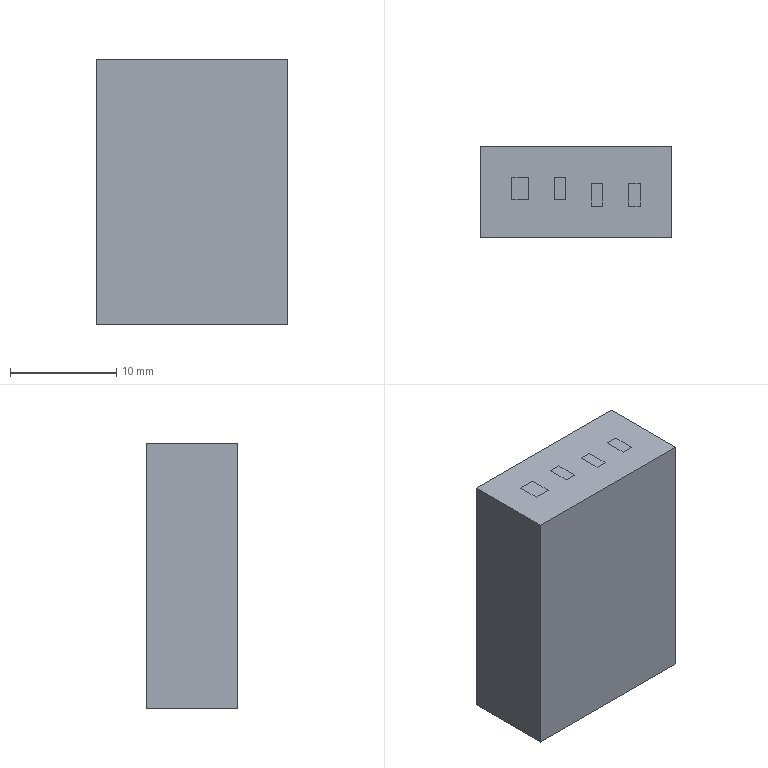Part | NX | features BREP 2 | 2 solids | 48 faces | box 18.008 x 8.593 x 25 mm | volume 6543 mm3 | plane 48
STEP:
#1=CARTESIAN_POINT('',(-9.004,-4.296,-25.6));
#2=VERTEX_POINT('',#1);
#3=CARTESIAN_POINT('',(-9.004,4.296,-25.6));
#4=VERTEX_POINT('',#3);
#5=CARTESIAN_POINT('',(-9.004,-4.296,-25.6));
#6=DIRECTION('',(0.,1.,0.));
#7=VECTOR('',#6,1000.);
#8=LINE('',#5,#7);
#9=EDGE_CURVE('',#2,#4,#8,.T.);
#10=ORIENTED_EDGE('',*,*,#9,.T.);
#11=CARTESIAN_POINT('',(9.004,4.296,-25.6));
#12=VERTEX_POINT('',#11);
#13=CARTESIAN_POINT('',(-9.004,4.296,-25.6));
#14=DIRECTION('',(1.,0.,0.));
#15=VECTOR('',#14,1000.);
#16=LINE('',#13,#15);
#17=EDGE_CURVE('',#4,#12,#16,.T.);
#18=ORIENTED_EDGE('',*,*,#17,.T.);
#19=CARTESIAN_POINT('',(9.004,-4.296,-25.6));
#20=VERTEX_POINT('',#19);
#21=CARTESIAN_POINT('',(9.004,4.296,-25.6));
#22=DIRECTION('',(0.,-1.,0.));
#23=VECTOR('',#22,1000.);
#24=LINE('',#21,#23);
#25=EDGE_CURVE('',#12,#20,#24,.T.);
#26=ORIENTED_EDGE('',*,*,#25,.T.);
#27=CARTESIAN_POINT('',(9.004,-4.296,-25.6));
#28=DIRECTION('',(-1.,0.,0.));
#29=VECTOR('',#28,1000.);
#30=LINE('',#27,#29);
#31=EDGE_CURVE('',#20,#2,#30,.T.);
#32=ORIENTED_EDGE('',*,*,#31,.T.);
#33=EDGE_LOOP('',(#10,#18,#26,#32));
#34=FACE_BOUND('',#33,.T.);
#35=CARTESIAN_POINT('',(7.054,1.754,-25.6));
#36=VERTEX_POINT('',#35);
#37=CARTESIAN_POINT('',(3.934,1.754,-25.6));
#38=VERTEX_POINT('',#37);
#39=CARTESIAN_POINT('',(-5.046,1.754,-25.6));
#40=DIRECTION('',(-1.,0.,0.));
#41=VECTOR('',#40,1000.);
#42=LINE('',#39,#41);
#43=EDGE_CURVE('',#36,#38,#42,.T.);
#44=ORIENTED_EDGE('',*,*,#43,.T.);
#45=CARTESIAN_POINT('',(3.934,-2.346,-25.6));
#46=VERTEX_POINT('',#45);
#47=CARTESIAN_POINT('',(3.934,-10.383,-25.6));
#48=DIRECTION('',(0.,-1.,0.));
#49=VECTOR('',#48,1000.);
#50=LINE('',#47,#49);
#51=EDGE_CURVE('',#38,#46,#50,.T.);
#52=ORIENTED_EDGE('',*,*,#51,.T.);
#53=CARTESIAN_POINT('',(7.054,-2.346,-25.6));
#54=VERTEX_POINT('',#53);
#55=CARTESIAN_POINT('',(-5.046,-2.346,-25.6));
#56=DIRECTION('',(1.,0.,0.));
#57=VECTOR('',#56,1000.);
#58=LINE('',#55,#57);
#59=EDGE_CURVE('',#46,#54,#58,.T.);
#60=ORIENTED_EDGE('',*,*,#59,.T.);
#61=CARTESIAN_POINT('',(7.054,1.396,-25.6));
#62=DIRECTION('',(0.,1.,0.));
#63=VECTOR('',#62,1000.);
#64=LINE('',#61,#63);
#65=EDGE_CURVE('',#54,#36,#64,.T.);
#66=ORIENTED_EDGE('',*,*,#65,.T.);
#67=EDGE_LOOP('',(#44,#52,#60,#66));
#68=FACE_BOUND('',#67,.T.);
#69=CARTESIAN_POINT('',(3.534,1.754,-25.6));
#70=VERTEX_POINT('',#69);
#71=CARTESIAN_POINT('',(0.454,1.754,-25.6));
#72=VERTEX_POINT('',#71);
#73=CARTESIAN_POINT('',(-5.046,1.754,-25.6));
#74=DIRECTION('',(-1.,0.,0.));
#75=VECTOR('',#74,1000.);
#76=LINE('',#73,#75);
#77=EDGE_CURVE('',#70,#72,#76,.T.);
#78=ORIENTED_EDGE('',*,*,#77,.T.);
#79=CARTESIAN_POINT('',(0.454,-2.346,-25.6));
#80=VERTEX_POINT('',#79);
#81=CARTESIAN_POINT('',(0.454,-1.296,-25.6));
#82=DIRECTION('',(0.,-1.,0.));
#83=VECTOR('',#82,1000.);
#84=LINE('',#81,#83);
#85=EDGE_CURVE('',#72,#80,#84,.T.);
#86=ORIENTED_EDGE('',*,*,#85,.T.);
#87=CARTESIAN_POINT('',(3.534,-2.346,-25.6));
#88=VERTEX_POINT('',#87);
#89=CARTESIAN_POINT('',(-5.046,-2.346,-25.6));
#90=DIRECTION('',(1.,0.,0.));
#91=VECTOR('',#90,1000.);
#92=LINE('',#89,#91);
#93=EDGE_CURVE('',#80,#88,#92,.T.);
#94=ORIENTED_EDGE('',*,*,#93,.T.);
#95=CARTESIAN_POINT('',(3.534,1.396,-25.6));
#96=DIRECTION('',(0.,1.,0.));
#97=VECTOR('',#96,1000.);
#98=LINE('',#95,#97);
#99=EDGE_CURVE('',#88,#70,#98,.T.);
#100=ORIENTED_EDGE('',*,*,#99,.T.);
#101=EDGE_LOOP('',(#78,#86,#94,#100));
#102=FACE_BOUND('',#101,.T.);
#103=CARTESIAN_POINT('',(0.04599,-1.754,-25.6));
#104=VERTEX_POINT('',#103);
#105=CARTESIAN_POINT('',(0.04599,2.346,-25.6));
#106=VERTEX_POINT('',#105);
#107=CARTESIAN_POINT('',(0.04599,4.296,-25.6));
#108=DIRECTION('',(0.,1.,0.));
#109=VECTOR('',#108,1000.);
#110=LINE('',#107,#109);
#111=EDGE_CURVE('',#104,#106,#110,.T.);
#112=ORIENTED_EDGE('',*,*,#111,.T.);
#113=CARTESIAN_POINT('',(-3.054,2.346,-25.6));
#114=VERTEX_POINT('',#113);
#115=CARTESIAN_POINT('',(-5.046,2.346,-25.6));
#116=DIRECTION('',(-1.,0.,0.));
#117=VECTOR('',#116,1000.);
#118=LINE('',#115,#117);
#119=EDGE_CURVE('',#106,#114,#118,.T.);
#120=ORIENTED_EDGE('',*,*,#119,.T.);
#121=CARTESIAN_POINT('',(-3.054,-1.754,-25.6));
#122=VERTEX_POINT('',#121);
#123=CARTESIAN_POINT('',(-3.054,-1.296,-25.6));
#124=DIRECTION('',(0.,-1.,0.));
#125=VECTOR('',#124,1000.);
#126=LINE('',#123,#125);
#127=EDGE_CURVE('',#114,#122,#126,.T.);
#128=ORIENTED_EDGE('',*,*,#127,.T.);
#129=CARTESIAN_POINT('',(-5.046,-1.754,-25.6));
#130=DIRECTION('',(1.,0.,0.));
#131=VECTOR('',#130,1000.);
#132=LINE('',#129,#131);
#133=EDGE_CURVE('',#122,#104,#132,.T.);
#134=ORIENTED_EDGE('',*,*,#133,.T.);
#135=EDGE_LOOP('',(#112,#120,#128,#134));
#136=FACE_BOUND('',#135,.T.);
#137=CARTESIAN_POINT('',(-3.454,-1.754,-25.6));
#138=VERTEX_POINT('',#137);
#139=CARTESIAN_POINT('',(-3.454,2.346,-25.6));
#140=VERTEX_POINT('',#139);
#141=CARTESIAN_POINT('',(-3.454,4.296,-25.6));
#142=DIRECTION('',(0.,1.,0.));
#143=VECTOR('',#142,1000.);
#144=LINE('',#141,#143);
#145=EDGE_CURVE('',#138,#140,#144,.T.);
#146=ORIENTED_EDGE('',*,*,#145,.T.);
#147=CARTESIAN_POINT('',(-7.054,2.346,-25.6));
#148=VERTEX_POINT('',#147);
#149=CARTESIAN_POINT('',(-5.046,2.346,-25.6));
#150=DIRECTION('',(-1.,0.,0.));
#151=VECTOR('',#150,1000.);
#152=LINE('',#149,#151);
#153=EDGE_CURVE('',#140,#148,#152,.T.);
#154=ORIENTED_EDGE('',*,*,#153,.T.);
#155=CARTESIAN_POINT('',(-7.054,-1.754,-25.6));
#156=VERTEX_POINT('',#155);
#157=CARTESIAN_POINT('',(-7.054,-1.196,-25.6));
#158=DIRECTION('',(0.,-1.,0.));
#159=VECTOR('',#158,1000.);
#160=LINE('',#157,#159);
#161=EDGE_CURVE('',#148,#156,#160,.T.);
#162=ORIENTED_EDGE('',*,*,#161,.T.);
#163=CARTESIAN_POINT('',(-5.046,-1.754,-25.6));
#164=DIRECTION('',(1.,0.,0.));
#165=VECTOR('',#164,1000.);
#166=LINE('',#163,#165);
#167=EDGE_CURVE('',#156,#138,#166,.T.);
#168=ORIENTED_EDGE('',*,*,#167,.T.);
#169=EDGE_LOOP('',(#146,#154,#162,#168));
#170=FACE_BOUND('',#169,.T.);
#171=CARTESIAN_POINT('',(0.,0.,-25.6));
#172=DIRECTION('',(0.,0.,-1.));
#173=DIRECTION('',(1.,0.,0.));
#174=AXIS2_PLACEMENT_3D('',#171,#172,#173);
#175=PLANE('',#174);
#176=ADVANCED_FACE('',(#34,#68,#102,#136,#170),#175,.T.);
#177=CARTESIAN_POINT('',(-0.954,1.346,-0.6));
#178=VERTEX_POINT('',#177);
#179=CARTESIAN_POINT('',(-2.054,1.346,-0.6));
#180=VERTEX_POINT('',#179);
#181=CARTESIAN_POINT('',(-5.046,1.346,-0.6));
#182=DIRECTION('',(-1.,0.,0.));
#183=VECTOR('',#182,1000.);
#184=LINE('',#181,#183);
#185=EDGE_CURVE('',#178,#180,#184,.T.);
#186=ORIENTED_EDGE('',*,*,#185,.F.);
#187=CARTESIAN_POINT('',(-0.954,-0.7536,-0.6));
#188=VERTEX_POINT('',#187);
#189=CARTESIAN_POINT('',(-0.954,4.296,-0.6));
#190=DIRECTION('',(0.,1.,0.));
#191=VECTOR('',#190,1000.);
#192=LINE('',#189,#191);
#193=EDGE_CURVE('',#188,#178,#192,.T.);
#194=ORIENTED_EDGE('',*,*,#193,.F.);
#195=CARTESIAN_POINT('',(-2.054,-0.7536,-0.6));
#196=VERTEX_POINT('',#195);
#197=CARTESIAN_POINT('',(-5.046,-0.7536,-0.6));
#198=DIRECTION('',(1.,0.,0.));
#199=VECTOR('',#198,1000.);
#200=LINE('',#197,#199);
#201=EDGE_CURVE('',#196,#188,#200,.T.);
#202=ORIENTED_EDGE('',*,*,#201,.F.);
#203=CARTESIAN_POINT('',(-2.054,-1.296,-0.6));
#204=DIRECTION('',(0.,-1.,0.));
#205=VECTOR('',#204,1000.);
#206=LINE('',#203,#205);
#207=EDGE_CURVE('',#180,#196,#206,.T.);
#208=ORIENTED_EDGE('',*,*,#207,.F.);
#209=EDGE_LOOP('',(#186,#194,#202,#208));
#210=FACE_BOUND('',#209,.T.);
#211=CARTESIAN_POINT('',(-9.004,-4.296,-0.6));
#212=VERTEX_POINT('',#211);
#213=CARTESIAN_POINT('',(-9.004,4.296,-0.6));
#214=VERTEX_POINT('',#213);
#215=CARTESIAN_POINT('',(-9.004,-4.296,-0.6));
#216=DIRECTION('',(0.,1.,0.));
#217=VECTOR('',#216,1000.);
#218=LINE('',#215,#217);
#219=EDGE_CURVE('',#212,#214,#218,.T.);
#220=ORIENTED_EDGE('',*,*,#219,.F.);
#221=CARTESIAN_POINT('',(9.004,-4.296,-0.6));
#222=VERTEX_POINT('',#221);
#223=CARTESIAN_POINT('',(9.004,-4.296,-0.6));
#224=DIRECTION('',(-1.,0.,0.));
#225=VECTOR('',#224,1000.);
#226=LINE('',#223,#225);
#227=EDGE_CURVE('',#222,#212,#226,.T.);
#228=ORIENTED_EDGE('',*,*,#227,.F.);
#229=CARTESIAN_POINT('',(9.004,4.296,-0.6));
#230=VERTEX_POINT('',#229);
#231=CARTESIAN_POINT('',(9.004,4.296,-0.6));
#232=DIRECTION('',(0.,-1.,0.));
#233=VECTOR('',#232,1000.);
#234=LINE('',#231,#233);
#235=EDGE_CURVE('',#230,#222,#234,.T.);
#236=ORIENTED_EDGE('',*,*,#235,.F.);
#237=CARTESIAN_POINT('',(-9.004,4.296,-0.6));
#238=DIRECTION('',(1.,0.,0.));
#239=VECTOR('',#238,1000.);
#240=LINE('',#237,#239);
#241=EDGE_CURVE('',#214,#230,#240,.T.);
#242=ORIENTED_EDGE('',*,*,#241,.F.);
#243=EDGE_LOOP('',(#220,#228,#236,#242));
#244=FACE_BOUND('',#243,.T.);
#245=CARTESIAN_POINT('',(4.934,0.7536,-0.6));
#246=VERTEX_POINT('',#245);
#247=CARTESIAN_POINT('',(4.934,-1.346,-0.6));
#248=VERTEX_POINT('',#247);
#249=CARTESIAN_POINT('',(4.934,-10.383,-0.6));
#250=DIRECTION('',(0.,-1.,0.));
#251=VECTOR('',#250,1000.);
#252=LINE('',#249,#251);
#253=EDGE_CURVE('',#246,#248,#252,.T.);
#254=ORIENTED_EDGE('',*,*,#253,.F.);
#255=CARTESIAN_POINT('',(6.054,0.7536,-0.6));
#256=VERTEX_POINT('',#255);
#257=CARTESIAN_POINT('',(-5.046,0.7536,-0.6));
#258=DIRECTION('',(-1.,0.,0.));
#259=VECTOR('',#258,1000.);
#260=LINE('',#257,#259);
#261=EDGE_CURVE('',#256,#246,#260,.T.);
#262=ORIENTED_EDGE('',*,*,#261,.F.);
#263=CARTESIAN_POINT('',(6.054,-1.346,-0.6));
#264=VERTEX_POINT('',#263);
#265=CARTESIAN_POINT('',(6.054,1.396,-0.6));
#266=DIRECTION('',(0.,1.,0.));
#267=VECTOR('',#266,1000.);
#268=LINE('',#265,#267);
#269=EDGE_CURVE('',#264,#256,#268,.T.);
#270=ORIENTED_EDGE('',*,*,#269,.F.);
#271=CARTESIAN_POINT('',(-5.046,-1.346,-0.6));
#272=DIRECTION('',(1.,0.,0.));
#273=VECTOR('',#272,1000.);
#274=LINE('',#271,#273);
#275=EDGE_CURVE('',#248,#264,#274,.T.);
#276=ORIENTED_EDGE('',*,*,#275,.F.);
#277=EDGE_LOOP('',(#254,#262,#270,#276));
#278=FACE_BOUND('',#277,.T.);
#279=CARTESIAN_POINT('',(1.454,0.7536,-0.6));
#280=VERTEX_POINT('',#279);
#281=CARTESIAN_POINT('',(1.454,-1.346,-0.6));
#282=VERTEX_POINT('',#281);
#283=CARTESIAN_POINT('',(1.454,-1.296,-0.6));
#284=DIRECTION('',(0.,-1.,0.));
#285=VECTOR('',#284,1000.);
#286=LINE('',#283,#285);
#287=EDGE_CURVE('',#280,#282,#286,.T.);
#288=ORIENTED_EDGE('',*,*,#287,.F.);
#289=CARTESIAN_POINT('',(2.534,0.7536,-0.6));
#290=VERTEX_POINT('',#289);
#291=CARTESIAN_POINT('',(-5.046,0.7536,-0.6));
#292=DIRECTION('',(-1.,0.,0.));
#293=VECTOR('',#292,1000.);
#294=LINE('',#291,#293);
#295=EDGE_CURVE('',#290,#280,#294,.T.);
#296=ORIENTED_EDGE('',*,*,#295,.F.);
#297=CARTESIAN_POINT('',(2.534,-1.346,-0.6));
#298=VERTEX_POINT('',#297);
#299=CARTESIAN_POINT('',(2.534,1.396,-0.6));
#300=DIRECTION('',(0.,1.,0.));
#301=VECTOR('',#300,1000.);
#302=LINE('',#299,#301);
#303=EDGE_CURVE('',#298,#290,#302,.T.);
#304=ORIENTED_EDGE('',*,*,#303,.F.);
#305=CARTESIAN_POINT('',(-5.046,-1.346,-0.6));
#306=DIRECTION('',(1.,0.,0.));
#307=VECTOR('',#306,1000.);
#308=LINE('',#305,#307);
#309=EDGE_CURVE('',#282,#298,#308,.T.);
#310=ORIENTED_EDGE('',*,*,#309,.F.);
#311=EDGE_LOOP('',(#288,#296,#304,#310));
#312=FACE_BOUND('',#311,.T.);
#313=CARTESIAN_POINT('',(-4.454,1.346,-0.6));
#314=VERTEX_POINT('',#313);
#315=CARTESIAN_POINT('',(-6.054,1.346,-0.6));
#316=VERTEX_POINT('',#315);
#317=CARTESIAN_POINT('',(-5.046,1.346,-0.6));
#318=DIRECTION('',(-1.,0.,0.));
#319=VECTOR('',#318,1000.);
#320=LINE('',#317,#319);
#321=EDGE_CURVE('',#314,#316,#320,.T.);
#322=ORIENTED_EDGE('',*,*,#321,.F.);
#323=CARTESIAN_POINT('',(-4.454,-0.7536,-0.6));
#324=VERTEX_POINT('',#323);
#325=CARTESIAN_POINT('',(-4.454,4.296,-0.6));
#326=DIRECTION('',(0.,1.,0.));
#327=VECTOR('',#326,1000.);
#328=LINE('',#325,#327);
#329=EDGE_CURVE('',#324,#314,#328,.T.);
#330=ORIENTED_EDGE('',*,*,#329,.F.);
#331=CARTESIAN_POINT('',(-6.054,-0.7536,-0.6));
#332=VERTEX_POINT('',#331);
#333=CARTESIAN_POINT('',(-5.046,-0.7536,-0.6));
#334=DIRECTION('',(1.,0.,0.));
#335=VECTOR('',#334,1000.);
#336=LINE('',#333,#335);
#337=EDGE_CURVE('',#332,#324,#336,.T.);
#338=ORIENTED_EDGE('',*,*,#337,.F.);
#339=CARTESIAN_POINT('',(-6.054,-1.196,-0.6));
#340=DIRECTION('',(0.,-1.,0.));
#341=VECTOR('',#340,1000.);
#342=LINE('',#339,#341);
#343=EDGE_CURVE('',#316,#332,#342,.T.);
#344=ORIENTED_EDGE('',*,*,#343,.F.);
#345=EDGE_LOOP('',(#322,#330,#338,#344));
#346=FACE_BOUND('',#345,.T.);
#347=CARTESIAN_POINT('',(0.,0.,-0.6));
#348=DIRECTION('',(0.,0.,-1.));
#349=DIRECTION('',(1.,0.,0.));
#350=AXIS2_PLACEMENT_3D('',#347,#348,#349);
#351=PLANE('',#350);
#352=ADVANCED_FACE('',(#210,#244,#278,#312,#346),#351,.F.);
#353=ORIENTED_EDGE('',*,*,#219,.T.);
#354=CARTESIAN_POINT('',(-9.004,4.296,-25.6));
#355=DIRECTION('',(0.,0.,1.));
#356=VECTOR('',#355,1000.);
#357=LINE('',#354,#356);
#358=EDGE_CURVE('',#4,#214,#357,.T.);
#359=ORIENTED_EDGE('',*,*,#358,.F.);
#360=ORIENTED_EDGE('',*,*,#9,.F.);
#361=CARTESIAN_POINT('',(-9.004,-4.296,-25.6));
#362=DIRECTION('',(0.,0.,1.));
#363=VECTOR('',#362,1000.);
#364=LINE('',#361,#363);
#365=EDGE_CURVE('',#2,#212,#364,.T.);
#366=ORIENTED_EDGE('',*,*,#365,.T.);
#367=EDGE_LOOP('',(#353,#359,#360,#366));
#368=FACE_BOUND('',#367,.T.);
#369=CARTESIAN_POINT('',(-9.004,-4.296,-25.6));
#370=DIRECTION('',(1.,0.,0.));
#371=DIRECTION('',(0.,0.,1.));
#372=AXIS2_PLACEMENT_3D('',#369,#370,#371);
#373=PLANE('',#372);
#374=ADVANCED_FACE('',(#368),#373,.F.);
#375=ORIENTED_EDGE('',*,*,#241,.T.);
#376=CARTESIAN_POINT('',(9.004,4.296,-25.6));
#377=DIRECTION('',(0.,0.,1.));
#378=VECTOR('',#377,1000.);
#379=LINE('',#376,#378);
#380=EDGE_CURVE('',#12,#230,#379,.T.);
#381=ORIENTED_EDGE('',*,*,#380,.F.);
#382=ORIENTED_EDGE('',*,*,#17,.F.);
#383=ORIENTED_EDGE('',*,*,#358,.T.);
#384=EDGE_LOOP('',(#375,#381,#382,#383));
#385=FACE_BOUND('',#384,.T.);
#386=CARTESIAN_POINT('',(-9.004,4.296,-25.6));
#387=DIRECTION('',(0.,-1.,0.));
#388=DIRECTION('',(-1.,0.,0.));
#389=AXIS2_PLACEMENT_3D('',#386,#387,#388);
#390=PLANE('',#389);
#391=ADVANCED_FACE('',(#385),#390,.F.);
#392=ORIENTED_EDGE('',*,*,#235,.T.);
#393=CARTESIAN_POINT('',(9.004,-4.296,-25.6));
#394=DIRECTION('',(0.,0.,1.));
#395=VECTOR('',#394,1000.);
#396=LINE('',#393,#395);
#397=EDGE_CURVE('',#20,#222,#396,.T.);
#398=ORIENTED_EDGE('',*,*,#397,.F.);
#399=ORIENTED_EDGE('',*,*,#25,.F.);
#400=ORIENTED_EDGE('',*,*,#380,.T.);
#401=EDGE_LOOP('',(#392,#398,#399,#400));
#402=FACE_BOUND('',#401,.T.);
#403=CARTESIAN_POINT('',(9.004,4.296,-25.6));
#404=DIRECTION('',(-1.,0.,0.));
#405=DIRECTION('',(0.,1.,0.));
#406=AXIS2_PLACEMENT_3D('',#403,#404,#405);
#407=PLANE('',#406);
#408=ADVANCED_FACE('',(#402),#407,.F.);
#409=ORIENTED_EDGE('',*,*,#227,.T.);
#410=ORIENTED_EDGE('',*,*,#365,.F.);
#411=ORIENTED_EDGE('',*,*,#31,.F.);
#412=ORIENTED_EDGE('',*,*,#397,.T.);
#413=EDGE_LOOP('',(#409,#410,#411,#412));
#414=FACE_BOUND('',#413,.T.);
#415=CARTESIAN_POINT('',(9.004,-4.296,-25.6));
#416=DIRECTION('',(0.,1.,0.));
#417=DIRECTION('',(1.,0.,0.));
#418=AXIS2_PLACEMENT_3D('',#415,#416,#417);
#419=PLANE('',#418);
#420=ADVANCED_FACE('',(#414),#419,.F.);
#421=CARTESIAN_POINT('',(6.054,0.7536,-3.6));
#422=VERTEX_POINT('',#421);
#423=CARTESIAN_POINT('',(6.054,0.7536,0.));
#424=DIRECTION('',(0.,0.,-1.));
#425=VECTOR('',#424,1000.);
#426=LINE('',#423,#425);
#427=EDGE_CURVE('',#256,#422,#426,.T.);
#428=ORIENTED_EDGE('',*,*,#427,.T.);
#429=CARTESIAN_POINT('',(6.054,-1.346,-3.6));
#430=VERTEX_POINT('',#429);
#431=CARTESIAN_POINT('',(6.054,1.396,-3.6));
#432=DIRECTION('',(0.,-1.,0.));
#433=VECTOR('',#432,1000.);
#434=LINE('',#431,#433);
#435=EDGE_CURVE('',#422,#430,#434,.T.);
#436=ORIENTED_EDGE('',*,*,#435,.T.);
#437=CARTESIAN_POINT('',(6.054,-1.346,0.));
#438=DIRECTION('',(0.,0.,-1.));
#439=VECTOR('',#438,1000.);
#440=LINE('',#437,#439);
#441=EDGE_CURVE('',#264,#430,#440,.T.);
#442=ORIENTED_EDGE('',*,*,#441,.F.);
#443=ORIENTED_EDGE('',*,*,#269,.T.);
#444=EDGE_LOOP('',(#428,#436,#442,#443));
#445=FACE_BOUND('',#444,.T.);
#446=CARTESIAN_POINT('',(6.054,1.396,0.));
#447=DIRECTION('',(-1.,0.,0.));
#448=DIRECTION('',(0.,1.,0.));
#449=AXIS2_PLACEMENT_3D('',#446,#447,#448);
#450=PLANE('',#449);
#451=ADVANCED_FACE('',(#445),#450,.T.);
#452=ORIENTED_EDGE('',*,*,#441,.T.);
#453=CARTESIAN_POINT('',(4.934,-1.346,-3.6));
#454=VERTEX_POINT('',#453);
#455=CARTESIAN_POINT('',(-5.046,-1.346,-3.6));
#456=DIRECTION('',(-1.,0.,0.));
#457=VECTOR('',#456,1000.);
#458=LINE('',#455,#457);
#459=EDGE_CURVE('',#430,#454,#458,.T.);
#460=ORIENTED_EDGE('',*,*,#459,.T.);
#461=CARTESIAN_POINT('',(4.934,-1.346,0.));
#462=DIRECTION('',(0.,0.,-1.));
#463=VECTOR('',#462,1000.);
#464=LINE('',#461,#463);
#465=EDGE_CURVE('',#248,#454,#464,.T.);
#466=ORIENTED_EDGE('',*,*,#465,.F.);
#467=ORIENTED_EDGE('',*,*,#275,.T.);
#468=EDGE_LOOP('',(#452,#460,#466,#467));
#469=FACE_BOUND('',#468,.T.);
#470=CARTESIAN_POINT('',(-5.046,-1.346,0.));
#471=DIRECTION('',(0.,-1.,0.));
#472=DIRECTION('',(-1.,0.,0.));
#473=AXIS2_PLACEMENT_3D('',#470,#471,#472);
#474=PLANE('',#473);
#475=ADVANCED_FACE('',(#469),#474,.F.);
#476=ORIENTED_EDGE('',*,*,#465,.T.);
#477=CARTESIAN_POINT('',(4.934,0.7536,-3.6));
#478=VERTEX_POINT('',#477);
#479=CARTESIAN_POINT('',(4.934,-10.383,-3.6));
#480=DIRECTION('',(0.,1.,0.));
#481=VECTOR('',#480,1000.);
#482=LINE('',#479,#481);
#483=EDGE_CURVE('',#454,#478,#482,.T.);
#484=ORIENTED_EDGE('',*,*,#483,.T.);
#485=CARTESIAN_POINT('',(4.934,0.7536,0.));
#486=DIRECTION('',(0.,0.,-1.));
#487=VECTOR('',#486,1000.);
#488=LINE('',#485,#487);
#489=EDGE_CURVE('',#246,#478,#488,.T.);
#490=ORIENTED_EDGE('',*,*,#489,.F.);
#491=ORIENTED_EDGE('',*,*,#253,.T.);
#492=EDGE_LOOP('',(#476,#484,#490,#491));
#493=FACE_BOUND('',#492,.T.);
#494=CARTESIAN_POINT('',(4.934,-10.383,0.));
#495=DIRECTION('',(1.,0.,0.));
#496=DIRECTION('',(0.,-1.,0.));
#497=AXIS2_PLACEMENT_3D('',#494,#495,#496);
#498=PLANE('',#497);
#499=ADVANCED_FACE('',(#493),#498,.T.);
#500=CARTESIAN_POINT('',(-5.046,0.7536,-3.6));
#501=DIRECTION('',(1.,0.,0.));
#502=VECTOR('',#501,1000.);
#503=LINE('',#500,#502);
#504=EDGE_CURVE('',#478,#422,#503,.T.);
#505=ORIENTED_EDGE('',*,*,#504,.T.);
#506=ORIENTED_EDGE('',*,*,#427,.F.);
#507=ORIENTED_EDGE('',*,*,#261,.T.);
#508=ORIENTED_EDGE('',*,*,#489,.T.);
#509=EDGE_LOOP('',(#505,#506,#507,#508));
#510=FACE_BOUND('',#509,.T.);
#511=CARTESIAN_POINT('',(-5.046,0.7536,0.));
#512=DIRECTION('',(0.,-1.,0.));
#513=DIRECTION('',(-1.,0.,0.));
#514=AXIS2_PLACEMENT_3D('',#511,#512,#513);
#515=PLANE('',#514);
#516=ADVANCED_FACE('',(#510),#515,.T.);
#517=CARTESIAN_POINT('',(3.934,-2.346,-3.6));
#518=VERTEX_POINT('',#517);
#519=CARTESIAN_POINT('',(3.934,1.754,-3.6));
#520=VERTEX_POINT('',#519);
#521=CARTESIAN_POINT('',(3.934,-10.383,-3.6));
#522=DIRECTION('',(0.,1.,0.));
#523=VECTOR('',#522,1000.);
#524=LINE('',#521,#523);
#525=EDGE_CURVE('',#518,#520,#524,.T.);
#526=ORIENTED_EDGE('',*,*,#525,.T.);
#527=CARTESIAN_POINT('',(7.054,1.754,-3.6));
#528=VERTEX_POINT('',#527);
#529=CARTESIAN_POINT('',(-5.046,1.754,-3.6));
#530=DIRECTION('',(1.,0.,0.));
#531=VECTOR('',#530,1000.);
#532=LINE('',#529,#531);
#533=EDGE_CURVE('',#520,#528,#532,.T.);
#534=ORIENTED_EDGE('',*,*,#533,.T.);
#535=CARTESIAN_POINT('',(7.054,-2.346,-3.6));
#536=VERTEX_POINT('',#535);
#537=CARTESIAN_POINT('',(7.054,1.396,-3.6));
#538=DIRECTION('',(0.,-1.,0.));
#539=VECTOR('',#538,1000.);
#540=LINE('',#537,#539);
#541=EDGE_CURVE('',#528,#536,#540,.T.);
#542=ORIENTED_EDGE('',*,*,#541,.T.);
#543=CARTESIAN_POINT('',(-5.046,-2.346,-3.6));
#544=DIRECTION('',(-1.,0.,0.));
#545=VECTOR('',#544,1000.);
#546=LINE('',#543,#545);
#547=EDGE_CURVE('',#536,#518,#546,.T.);
#548=ORIENTED_EDGE('',*,*,#547,.T.);
#549=EDGE_LOOP('',(#526,#534,#542,#548));
#550=FACE_BOUND('',#549,.T.);
#551=ORIENTED_EDGE('',*,*,#459,.F.);
#552=ORIENTED_EDGE('',*,*,#435,.F.);
#553=ORIENTED_EDGE('',*,*,#504,.F.);
#554=ORIENTED_EDGE('',*,*,#483,.F.);
#555=EDGE_LOOP('',(#551,#552,#553,#554));
#556=FACE_BOUND('',#555,.T.);
#557=CARTESIAN_POINT('',(-5.046,-13.002,-3.6));
#558=DIRECTION('',(0.,0.,1.));
#559=DIRECTION('',(-1.,0.,0.));
#560=AXIS2_PLACEMENT_3D('',#557,#558,#559);
#561=PLANE('',#560);
#562=ADVANCED_FACE('',(#550,#556),#561,.F.);
#563=CARTESIAN_POINT('',(7.054,1.754,-3.6));
#564=DIRECTION('',(0.,0.,-1.));
#565=VECTOR('',#564,1000.);
#566=LINE('',#563,#565);
#567=EDGE_CURVE('',#528,#36,#566,.T.);
#568=ORIENTED_EDGE('',*,*,#567,.T.);
#569=ORIENTED_EDGE('',*,*,#65,.F.);
#570=CARTESIAN_POINT('',(7.054,-2.346,-3.6));
#571=DIRECTION('',(0.,0.,-1.));
#572=VECTOR('',#571,1000.);
#573=LINE('',#570,#572);
#574=EDGE_CURVE('',#536,#54,#573,.T.);
#575=ORIENTED_EDGE('',*,*,#574,.F.);
#576=ORIENTED_EDGE('',*,*,#541,.F.);
#577=EDGE_LOOP('',(#568,#569,#575,#576));
#578=FACE_BOUND('',#577,.T.);
#579=CARTESIAN_POINT('',(7.054,1.396,-3.6));
#580=DIRECTION('',(1.,0.,0.));
#581=DIRECTION('',(0.,-1.,0.));
#582=AXIS2_PLACEMENT_3D('',#579,#580,#581);
#583=PLANE('',#582);
#584=ADVANCED_FACE('',(#578),#583,.F.);
#585=ORIENTED_EDGE('',*,*,#574,.T.);
#586=ORIENTED_EDGE('',*,*,#59,.F.);
#587=CARTESIAN_POINT('',(3.934,-2.346,-3.6));
#588=DIRECTION('',(0.,0.,-1.));
#589=VECTOR('',#588,1000.);
#590=LINE('',#587,#589);
#591=EDGE_CURVE('',#518,#46,#590,.T.);
#592=ORIENTED_EDGE('',*,*,#591,.F.);
#593=ORIENTED_EDGE('',*,*,#547,.F.);
#594=EDGE_LOOP('',(#585,#586,#592,#593));
#595=FACE_BOUND('',#594,.T.);
#596=CARTESIAN_POINT('',(-5.046,-2.346,-3.6));
#597=DIRECTION('',(0.,1.,0.));
#598=DIRECTION('',(1.,0.,0.));
#599=AXIS2_PLACEMENT_3D('',#596,#597,#598);
#600=PLANE('',#599);
#601=ADVANCED_FACE('',(#595),#600,.T.);
#602=ORIENTED_EDGE('',*,*,#591,.T.);
#603=ORIENTED_EDGE('',*,*,#51,.F.);
#604=CARTESIAN_POINT('',(3.934,1.754,-3.6));
#605=DIRECTION('',(0.,0.,-1.));
#606=VECTOR('',#605,1000.);
#607=LINE('',#604,#606);
#608=EDGE_CURVE('',#520,#38,#607,.T.);
#609=ORIENTED_EDGE('',*,*,#608,.F.);
#610=ORIENTED_EDGE('',*,*,#525,.F.);
#611=EDGE_LOOP('',(#602,#603,#609,#610));
#612=FACE_BOUND('',#611,.T.);
#613=CARTESIAN_POINT('',(3.934,-10.383,-3.6));
#614=DIRECTION('',(-1.,0.,0.));
#615=DIRECTION('',(0.,1.,0.));
#616=AXIS2_PLACEMENT_3D('',#613,#614,#615);
#617=PLANE('',#616);
#618=ADVANCED_FACE('',(#612),#617,.F.);
#619=ORIENTED_EDGE('',*,*,#43,.F.);
#620=ORIENTED_EDGE('',*,*,#567,.F.);
#621=ORIENTED_EDGE('',*,*,#533,.F.);
#622=ORIENTED_EDGE('',*,*,#608,.T.);
#623=EDGE_LOOP('',(#619,#620,#621,#622));
#624=FACE_BOUND('',#623,.T.);
#625=CARTESIAN_POINT('',(-5.046,1.754,-3.6));
#626=DIRECTION('',(0.,1.,0.));
#627=DIRECTION('',(1.,0.,0.));
#628=AXIS2_PLACEMENT_3D('',#625,#626,#627);
#629=PLANE('',#628);
#630=ADVANCED_FACE('',(#624),#629,.F.);
#631=CARTESIAN_POINT('',(2.534,0.7536,-3.6));
#632=VERTEX_POINT('',#631);
#633=CARTESIAN_POINT('',(2.534,0.7536,0.));
#634=DIRECTION('',(0.,0.,-1.));
#635=VECTOR('',#634,1000.);
#636=LINE('',#633,#635);
#637=EDGE_CURVE('',#290,#632,#636,.T.);
#638=ORIENTED_EDGE('',*,*,#637,.T.);
#639=CARTESIAN_POINT('',(2.534,-1.346,-3.6));
#640=VERTEX_POINT('',#639);
#641=CARTESIAN_POINT('',(2.534,1.396,-3.6));
#642=DIRECTION('',(0.,-1.,0.));
#643=VECTOR('',#642,1000.);
#644=LINE('',#641,#643);
#645=EDGE_CURVE('',#632,#640,#644,.T.);
#646=ORIENTED_EDGE('',*,*,#645,.T.);
#647=CARTESIAN_POINT('',(2.534,-1.346,0.));
#648=DIRECTION('',(0.,0.,-1.));
#649=VECTOR('',#648,1000.);
#650=LINE('',#647,#649);
#651=EDGE_CURVE('',#298,#640,#650,.T.);
#652=ORIENTED_EDGE('',*,*,#651,.F.);
#653=ORIENTED_EDGE('',*,*,#303,.T.);
#654=EDGE_LOOP('',(#638,#646,#652,#653));
#655=FACE_BOUND('',#654,.T.);
#656=CARTESIAN_POINT('',(2.534,1.396,0.));
#657=DIRECTION('',(-1.,0.,0.));
#658=DIRECTION('',(0.,1.,0.));
#659=AXIS2_PLACEMENT_3D('',#656,#657,#658);
#660=PLANE('',#659);
#661=ADVANCED_FACE('',(#655),#660,.T.);
#662=ORIENTED_EDGE('',*,*,#651,.T.);
#663=CARTESIAN_POINT('',(1.454,-1.346,-3.6));
#664=VERTEX_POINT('',#663);
#665=CARTESIAN_POINT('',(-5.046,-1.346,-3.6));
#666=DIRECTION('',(-1.,0.,0.));
#667=VECTOR('',#666,1000.);
#668=LINE('',#665,#667);
#669=EDGE_CURVE('',#640,#664,#668,.T.);
#670=ORIENTED_EDGE('',*,*,#669,.T.);
#671=CARTESIAN_POINT('',(1.454,-1.346,0.));
#672=DIRECTION('',(0.,0.,-1.));
#673=VECTOR('',#672,1000.);
#674=LINE('',#671,#673);
#675=EDGE_CURVE('',#282,#664,#674,.T.);
#676=ORIENTED_EDGE('',*,*,#675,.F.);
#677=ORIENTED_EDGE('',*,*,#309,.T.);
#678=EDGE_LOOP('',(#662,#670,#676,#677));
#679=FACE_BOUND('',#678,.T.);
#680=CARTESIAN_POINT('',(-5.046,-1.346,0.));
#681=DIRECTION('',(0.,-1.,0.));
#682=DIRECTION('',(-1.,0.,0.));
#683=AXIS2_PLACEMENT_3D('',#680,#681,#682);
#684=PLANE('',#683);
#685=ADVANCED_FACE('',(#679),#684,.F.);
#686=ORIENTED_EDGE('',*,*,#675,.T.);
#687=CARTESIAN_POINT('',(1.454,0.7536,-3.6));
#688=VERTEX_POINT('',#687);
#689=CARTESIAN_POINT('',(1.454,-1.296,-3.6));
#690=DIRECTION('',(0.,1.,0.));
#691=VECTOR('',#690,1000.);
#692=LINE('',#689,#691);
#693=EDGE_CURVE('',#664,#688,#692,.T.);
#694=ORIENTED_EDGE('',*,*,#693,.T.);
#695=CARTESIAN_POINT('',(1.454,0.7536,0.));
#696=DIRECTION('',(0.,0.,-1.));
#697=VECTOR('',#696,1000.);
#698=LINE('',#695,#697);
#699=EDGE_CURVE('',#280,#688,#698,.T.);
#700=ORIENTED_EDGE('',*,*,#699,.F.);
#701=ORIENTED_EDGE('',*,*,#287,.T.);
#702=EDGE_LOOP('',(#686,#694,#700,#701));
#703=FACE_BOUND('',#702,.T.);
#704=CARTESIAN_POINT('',(1.454,-1.296,0.));
#705=DIRECTION('',(1.,0.,0.));
#706=DIRECTION('',(0.,-1.,0.));
#707=AXIS2_PLACEMENT_3D('',#704,#705,#706);
#708=PLANE('',#707);
#709=ADVANCED_FACE('',(#703),#708,.T.);
#710=CARTESIAN_POINT('',(-5.046,0.7536,-3.6));
#711=DIRECTION('',(1.,0.,0.));
#712=VECTOR('',#711,1000.);
#713=LINE('',#710,#712);
#714=EDGE_CURVE('',#688,#632,#713,.T.);
#715=ORIENTED_EDGE('',*,*,#714,.T.);
#716=ORIENTED_EDGE('',*,*,#637,.F.);
#717=ORIENTED_EDGE('',*,*,#295,.T.);
#718=ORIENTED_EDGE('',*,*,#699,.T.);
#719=EDGE_LOOP('',(#715,#716,#717,#718));
#720=FACE_BOUND('',#719,.T.);
#721=CARTESIAN_POINT('',(-5.046,0.7536,0.));
#722=DIRECTION('',(0.,-1.,0.));
#723=DIRECTION('',(-1.,0.,0.));
#724=AXIS2_PLACEMENT_3D('',#721,#722,#723);
#725=PLANE('',#724);
#726=ADVANCED_FACE('',(#720),#725,.T.);
#727=CARTESIAN_POINT('',(0.454,-2.346,-3.6));
#728=VERTEX_POINT('',#727);
#729=CARTESIAN_POINT('',(0.454,1.754,-3.6));
#730=VERTEX_POINT('',#729);
#731=CARTESIAN_POINT('',(0.454,-1.296,-3.6));
#732=DIRECTION('',(0.,1.,0.));
#733=VECTOR('',#732,1000.);
#734=LINE('',#731,#733);
#735=EDGE_CURVE('',#728,#730,#734,.T.);
#736=ORIENTED_EDGE('',*,*,#735,.T.);
#737=CARTESIAN_POINT('',(3.534,1.754,-3.6));
#738=VERTEX_POINT('',#737);
#739=CARTESIAN_POINT('',(-5.046,1.754,-3.6));
#740=DIRECTION('',(1.,0.,0.));
#741=VECTOR('',#740,1000.);
#742=LINE('',#739,#741);
#743=EDGE_CURVE('',#730,#738,#742,.T.);
#744=ORIENTED_EDGE('',*,*,#743,.T.);
#745=CARTESIAN_POINT('',(3.534,-2.346,-3.6));
#746=VERTEX_POINT('',#745);
#747=CARTESIAN_POINT('',(3.534,1.396,-3.6));
#748=DIRECTION('',(0.,-1.,0.));
#749=VECTOR('',#748,1000.);
#750=LINE('',#747,#749);
#751=EDGE_CURVE('',#738,#746,#750,.T.);
#752=ORIENTED_EDGE('',*,*,#751,.T.);
#753=CARTESIAN_POINT('',(-5.046,-2.346,-3.6));
#754=DIRECTION('',(-1.,0.,0.));
#755=VECTOR('',#754,1000.);
#756=LINE('',#753,#755);
#757=EDGE_CURVE('',#746,#728,#756,.T.);
#758=ORIENTED_EDGE('',*,*,#757,.T.);
#759=EDGE_LOOP('',(#736,#744,#752,#758));
#760=FACE_BOUND('',#759,.T.);
#761=ORIENTED_EDGE('',*,*,#669,.F.);
#762=ORIENTED_EDGE('',*,*,#645,.F.);
#763=ORIENTED_EDGE('',*,*,#714,.F.);
#764=ORIENTED_EDGE('',*,*,#693,.F.);
#765=EDGE_LOOP('',(#761,#762,#763,#764));
#766=FACE_BOUND('',#765,.T.);
#767=CARTESIAN_POINT('',(-5.046,-13.002,-3.6));
#768=DIRECTION('',(0.,0.,1.));
#769=DIRECTION('',(-1.,0.,0.));
#770=AXIS2_PLACEMENT_3D('',#767,#768,#769);
#771=PLANE('',#770);
#772=ADVANCED_FACE('',(#760,#766),#771,.F.);
#773=CARTESIAN_POINT('',(3.534,1.754,-3.6));
#774=DIRECTION('',(0.,0.,-1.));
#775=VECTOR('',#774,1000.);
#776=LINE('',#773,#775);
#777=EDGE_CURVE('',#738,#70,#776,.T.);
#778=ORIENTED_EDGE('',*,*,#777,.T.);
#779=ORIENTED_EDGE('',*,*,#99,.F.);
#780=CARTESIAN_POINT('',(3.534,-2.346,-3.6));
#781=DIRECTION('',(0.,0.,-1.));
#782=VECTOR('',#781,1000.);
#783=LINE('',#780,#782);
#784=EDGE_CURVE('',#746,#88,#783,.T.);
#785=ORIENTED_EDGE('',*,*,#784,.F.);
#786=ORIENTED_EDGE('',*,*,#751,.F.);
#787=EDGE_LOOP('',(#778,#779,#785,#786));
#788=FACE_BOUND('',#787,.T.);
#789=CARTESIAN_POINT('',(3.534,1.396,-3.6));
#790=DIRECTION('',(1.,0.,0.));
#791=DIRECTION('',(0.,-1.,0.));
#792=AXIS2_PLACEMENT_3D('',#789,#790,#791);
#793=PLANE('',#792);
#794=ADVANCED_FACE('',(#788),#793,.F.);
#795=ORIENTED_EDGE('',*,*,#784,.T.);
#796=ORIENTED_EDGE('',*,*,#93,.F.);
#797=CARTESIAN_POINT('',(0.454,-2.346,-3.6));
#798=DIRECTION('',(0.,0.,-1.));
#799=VECTOR('',#798,1000.);
#800=LINE('',#797,#799);
#801=EDGE_CURVE('',#728,#80,#800,.T.);
#802=ORIENTED_EDGE('',*,*,#801,.F.);
#803=ORIENTED_EDGE('',*,*,#757,.F.);
#804=EDGE_LOOP('',(#795,#796,#802,#803));
#805=FACE_BOUND('',#804,.T.);
#806=CARTESIAN_POINT('',(-5.046,-2.346,-3.6));
#807=DIRECTION('',(0.,1.,0.));
#808=DIRECTION('',(1.,0.,0.));
#809=AXIS2_PLACEMENT_3D('',#806,#807,#808);
#810=PLANE('',#809);
#811=ADVANCED_FACE('',(#805),#810,.T.);
#812=ORIENTED_EDGE('',*,*,#801,.T.);
#813=ORIENTED_EDGE('',*,*,#85,.F.);
#814=CARTESIAN_POINT('',(0.454,1.754,-3.6));
#815=DIRECTION('',(0.,0.,-1.));
#816=VECTOR('',#815,1000.);
#817=LINE('',#814,#816);
#818=EDGE_CURVE('',#730,#72,#817,.T.);
#819=ORIENTED_EDGE('',*,*,#818,.F.);
#820=ORIENTED_EDGE('',*,*,#735,.F.);
#821=EDGE_LOOP('',(#812,#813,#819,#820));
#822=FACE_BOUND('',#821,.T.);
#823=CARTESIAN_POINT('',(0.454,-1.296,-3.6));
#824=DIRECTION('',(-1.,0.,0.));
#825=DIRECTION('',(0.,1.,0.));
#826=AXIS2_PLACEMENT_3D('',#823,#824,#825);
#827=PLANE('',#826);
#828=ADVANCED_FACE('',(#822),#827,.F.);
#829=ORIENTED_EDGE('',*,*,#77,.F.);
#830=ORIENTED_EDGE('',*,*,#777,.F.);
#831=ORIENTED_EDGE('',*,*,#743,.F.);
#832=ORIENTED_EDGE('',*,*,#818,.T.);
#833=EDGE_LOOP('',(#829,#830,#831,#832));
#834=FACE_BOUND('',#833,.T.);
#835=CARTESIAN_POINT('',(-5.046,1.754,-3.6));
#836=DIRECTION('',(0.,1.,0.));
#837=DIRECTION('',(1.,0.,0.));
#838=AXIS2_PLACEMENT_3D('',#835,#836,#837);
#839=PLANE('',#838);
#840=ADVANCED_FACE('',(#834),#839,.F.);
#841=CARTESIAN_POINT('',(-0.954,-0.7536,-3.6));
#842=VERTEX_POINT('',#841);
#843=CARTESIAN_POINT('',(-0.954,-0.7536,0.));
#844=DIRECTION('',(0.,0.,-1.));
#845=VECTOR('',#844,1000.);
#846=LINE('',#843,#845);
#847=EDGE_CURVE('',#188,#842,#846,.T.);
#848=ORIENTED_EDGE('',*,*,#847,.T.);
#849=CARTESIAN_POINT('',(-2.054,-0.7536,-3.6));
#850=VERTEX_POINT('',#849);
#851=CARTESIAN_POINT('',(-5.046,-0.7536,-3.6));
#852=DIRECTION('',(-1.,0.,0.));
#853=VECTOR('',#852,1000.);
#854=LINE('',#851,#853);
#855=EDGE_CURVE('',#842,#850,#854,.T.);
#856=ORIENTED_EDGE('',*,*,#855,.T.);
#857=CARTESIAN_POINT('',(-2.054,-0.7536,0.));
#858=DIRECTION('',(0.,0.,-1.));
#859=VECTOR('',#858,1000.);
#860=LINE('',#857,#859);
#861=EDGE_CURVE('',#196,#850,#860,.T.);
#862=ORIENTED_EDGE('',*,*,#861,.F.);
#863=ORIENTED_EDGE('',*,*,#201,.T.);
#864=EDGE_LOOP('',(#848,#856,#862,#863));
#865=FACE_BOUND('',#864,.T.);
#866=CARTESIAN_POINT('',(-5.046,-0.7536,0.));
#867=DIRECTION('',(0.,-1.,0.));
#868=DIRECTION('',(-1.,0.,0.));
#869=AXIS2_PLACEMENT_3D('',#866,#867,#868);
#870=PLANE('',#869);
#871=ADVANCED_FACE('',(#865),#870,.F.);
#872=ORIENTED_EDGE('',*,*,#861,.T.);
#873=CARTESIAN_POINT('',(-2.054,1.346,-3.6));
#874=VERTEX_POINT('',#873);
#875=CARTESIAN_POINT('',(-2.054,-1.296,-3.6));
#876=DIRECTION('',(0.,1.,0.));
#877=VECTOR('',#876,1000.);
#878=LINE('',#875,#877);
#879=EDGE_CURVE('',#850,#874,#878,.T.);
#880=ORIENTED_EDGE('',*,*,#879,.T.);
#881=CARTESIAN_POINT('',(-2.054,1.346,0.));
#882=DIRECTION('',(0.,0.,-1.));
#883=VECTOR('',#882,1000.);
#884=LINE('',#881,#883);
#885=EDGE_CURVE('',#180,#874,#884,.T.);
#886=ORIENTED_EDGE('',*,*,#885,.F.);
#887=ORIENTED_EDGE('',*,*,#207,.T.);
#888=EDGE_LOOP('',(#872,#880,#886,#887));
#889=FACE_BOUND('',#888,.T.);
#890=CARTESIAN_POINT('',(-2.054,-1.296,0.));
#891=DIRECTION('',(1.,0.,0.));
#892=DIRECTION('',(0.,-1.,0.));
#893=AXIS2_PLACEMENT_3D('',#890,#891,#892);
#894=PLANE('',#893);
#895=ADVANCED_FACE('',(#889),#894,.T.);
#896=ORIENTED_EDGE('',*,*,#885,.T.);
#897=CARTESIAN_POINT('',(-0.954,1.346,-3.6));
#898=VERTEX_POINT('',#897);
#899=CARTESIAN_POINT('',(-5.046,1.346,-3.6));
#900=DIRECTION('',(1.,0.,0.));
#901=VECTOR('',#900,1000.);
#902=LINE('',#899,#901);
#903=EDGE_CURVE('',#874,#898,#902,.T.);
#904=ORIENTED_EDGE('',*,*,#903,.T.);
#905=CARTESIAN_POINT('',(-0.954,1.346,0.));
#906=DIRECTION('',(0.,0.,-1.));
#907=VECTOR('',#906,1000.);
#908=LINE('',#905,#907);
#909=EDGE_CURVE('',#178,#898,#908,.T.);
#910=ORIENTED_EDGE('',*,*,#909,.F.);
#911=ORIENTED_EDGE('',*,*,#185,.T.);
#912=EDGE_LOOP('',(#896,#904,#910,#911));
#913=FACE_BOUND('',#912,.T.);
#914=CARTESIAN_POINT('',(-5.046,1.346,0.));
#915=DIRECTION('',(0.,-1.,0.));
#916=DIRECTION('',(-1.,0.,0.));
#917=AXIS2_PLACEMENT_3D('',#914,#915,#916);
#918=PLANE('',#917);
#919=ADVANCED_FACE('',(#913),#918,.T.);
#920=CARTESIAN_POINT('',(-0.954,4.296,-3.6));
#921=DIRECTION('',(0.,-1.,0.));
#922=VECTOR('',#921,1000.);
#923=LINE('',#920,#922);
#924=EDGE_CURVE('',#898,#842,#923,.T.);
#925=ORIENTED_EDGE('',*,*,#924,.T.);
#926=ORIENTED_EDGE('',*,*,#847,.F.);
#927=ORIENTED_EDGE('',*,*,#193,.T.);
#928=ORIENTED_EDGE('',*,*,#909,.T.);
#929=EDGE_LOOP('',(#925,#926,#927,#928));
#930=FACE_BOUND('',#929,.T.);
#931=CARTESIAN_POINT('',(-0.954,4.296,0.));
#932=DIRECTION('',(-1.,0.,0.));
#933=DIRECTION('',(0.,1.,0.));
#934=AXIS2_PLACEMENT_3D('',#931,#932,#933);
#935=PLANE('',#934);
#936=ADVANCED_FACE('',(#930),#935,.T.);
#937=CARTESIAN_POINT('',(-3.054,2.346,-3.6));
#938=VERTEX_POINT('',#937);
#939=CARTESIAN_POINT('',(0.04599,2.346,-3.6));
#940=VERTEX_POINT('',#939);
#941=CARTESIAN_POINT('',(-5.046,2.346,-3.6));
#942=DIRECTION('',(1.,0.,0.));
#943=VECTOR('',#942,1000.);
#944=LINE('',#941,#943);
#945=EDGE_CURVE('',#938,#940,#944,.T.);
#946=ORIENTED_EDGE('',*,*,#945,.T.);
#947=CARTESIAN_POINT('',(0.04599,-1.754,-3.6));
#948=VERTEX_POINT('',#947);
#949=CARTESIAN_POINT('',(0.04599,4.296,-3.6));
#950=DIRECTION('',(0.,-1.,0.));
#951=VECTOR('',#950,1000.);
#952=LINE('',#949,#951);
#953=EDGE_CURVE('',#940,#948,#952,.T.);
#954=ORIENTED_EDGE('',*,*,#953,.T.);
#955=CARTESIAN_POINT('',(-3.054,-1.754,-3.6));
#956=VERTEX_POINT('',#955);
#957=CARTESIAN_POINT('',(-5.046,-1.754,-3.6));
#958=DIRECTION('',(-1.,0.,0.));
#959=VECTOR('',#958,1000.);
#960=LINE('',#957,#959);
#961=EDGE_CURVE('',#948,#956,#960,.T.);
#962=ORIENTED_EDGE('',*,*,#961,.T.);
#963=CARTESIAN_POINT('',(-3.054,-1.296,-3.6));
#964=DIRECTION('',(0.,1.,0.));
#965=VECTOR('',#964,1000.);
#966=LINE('',#963,#965);
#967=EDGE_CURVE('',#956,#938,#966,.T.);
#968=ORIENTED_EDGE('',*,*,#967,.T.);
#969=EDGE_LOOP('',(#946,#954,#962,#968));
#970=FACE_BOUND('',#969,.T.);
#971=ORIENTED_EDGE('',*,*,#879,.F.);
#972=ORIENTED_EDGE('',*,*,#855,.F.);
#973=ORIENTED_EDGE('',*,*,#924,.F.);
#974=ORIENTED_EDGE('',*,*,#903,.F.);
#975=EDGE_LOOP('',(#971,#972,#973,#974));
#976=FACE_BOUND('',#975,.T.);
#977=CARTESIAN_POINT('',(-5.046,-13.002,-3.6));
#978=DIRECTION('',(0.,0.,1.));
#979=DIRECTION('',(-1.,0.,0.));
#980=AXIS2_PLACEMENT_3D('',#977,#978,#979);
#981=PLANE('',#980);
#982=ADVANCED_FACE('',(#970,#976),#981,.F.);
#983=CARTESIAN_POINT('',(0.04599,-1.754,-3.6));
#984=DIRECTION('',(0.,0.,-1.));
#985=VECTOR('',#984,1000.);
#986=LINE('',#983,#985);
#987=EDGE_CURVE('',#948,#104,#986,.T.);
#988=ORIENTED_EDGE('',*,*,#987,.T.);
#989=ORIENTED_EDGE('',*,*,#133,.F.);
#990=CARTESIAN_POINT('',(-3.054,-1.754,-3.6));
#991=DIRECTION('',(0.,0.,-1.));
#992=VECTOR('',#991,1000.);
#993=LINE('',#990,#992);
#994=EDGE_CURVE('',#956,#122,#993,.T.);
#995=ORIENTED_EDGE('',*,*,#994,.F.);
#996=ORIENTED_EDGE('',*,*,#961,.F.);
#997=EDGE_LOOP('',(#988,#989,#995,#996));
#998=FACE_BOUND('',#997,.T.);
#999=CARTESIAN_POINT('',(-5.046,-1.754,-3.6));
#1000=DIRECTION('',(0.,1.,0.));
#1001=DIRECTION('',(1.,0.,0.));
#1002=AXIS2_PLACEMENT_3D('',#999,#1000,#1001);
#1003=PLANE('',#1002);
#1004=ADVANCED_FACE('',(#998),#1003,.T.);
#1005=ORIENTED_EDGE('',*,*,#994,.T.);
#1006=ORIENTED_EDGE('',*,*,#127,.F.);
#1007=CARTESIAN_POINT('',(-3.054,2.346,-3.6));
#1008=DIRECTION('',(0.,0.,-1.));
#1009=VECTOR('',#1008,1000.);
#1010=LINE('',#1007,#1009);
#1011=EDGE_CURVE('',#938,#114,#1010,.T.);
#1012=ORIENTED_EDGE('',*,*,#1011,.F.);
#1013=ORIENTED_EDGE('',*,*,#967,.F.);
#1014=EDGE_LOOP('',(#1005,#1006,#1012,#1013));
#1015=FACE_BOUND('',#1014,.T.);
#1016=CARTESIAN_POINT('',(-3.054,-1.296,-3.6));
#1017=DIRECTION('',(-1.,0.,0.));
#1018=DIRECTION('',(0.,1.,0.));
#1019=AXIS2_PLACEMENT_3D('',#1016,#1017,#1018);
#1020=PLANE('',#1019);
#1021=ADVANCED_FACE('',(#1015),#1020,.F.);
#1022=ORIENTED_EDGE('',*,*,#1011,.T.);
#1023=ORIENTED_EDGE('',*,*,#119,.F.);
#1024=CARTESIAN_POINT('',(0.04599,2.346,-3.6));
#1025=DIRECTION('',(0.,0.,-1.));
#1026=VECTOR('',#1025,1000.);
#1027=LINE('',#1024,#1026);
#1028=EDGE_CURVE('',#940,#106,#1027,.T.);
#1029=ORIENTED_EDGE('',*,*,#1028,.F.);
#1030=ORIENTED_EDGE('',*,*,#945,.F.);
#1031=EDGE_LOOP('',(#1022,#1023,#1029,#1030));
#1032=FACE_BOUND('',#1031,.T.);
#1033=CARTESIAN_POINT('',(-5.046,2.346,-3.6));
#1034=DIRECTION('',(0.,1.,0.));
#1035=DIRECTION('',(1.,0.,0.));
#1036=AXIS2_PLACEMENT_3D('',#1033,#1034,#1035);
#1037=PLANE('',#1036);
#1038=ADVANCED_FACE('',(#1032),#1037,.F.);
#1039=ORIENTED_EDGE('',*,*,#111,.F.);
#1040=ORIENTED_EDGE('',*,*,#987,.F.);
#1041=ORIENTED_EDGE('',*,*,#953,.F.);
#1042=ORIENTED_EDGE('',*,*,#1028,.T.);
#1043=EDGE_LOOP('',(#1039,#1040,#1041,#1042));
#1044=FACE_BOUND('',#1043,.T.);
#1045=CARTESIAN_POINT('',(0.04599,4.296,-3.6));
#1046=DIRECTION('',(1.,0.,0.));
#1047=DIRECTION('',(0.,-1.,0.));
#1048=AXIS2_PLACEMENT_3D('',#1045,#1046,#1047);
#1049=PLANE('',#1048);
#1050=ADVANCED_FACE('',(#1044),#1049,.F.);
#1051=CARTESIAN_POINT('',(-4.454,-0.7536,-3.6));
#1052=VERTEX_POINT('',#1051);
#1053=CARTESIAN_POINT('',(-4.454,-0.7536,0.));
#1054=DIRECTION('',(0.,0.,-1.));
#1055=VECTOR('',#1054,1000.);
#1056=LINE('',#1053,#1055);
#1057=EDGE_CURVE('',#324,#1052,#1056,.T.);
#1058=ORIENTED_EDGE('',*,*,#1057,.T.);
#1059=CARTESIAN_POINT('',(-6.054,-0.7536,-3.6));
#1060=VERTEX_POINT('',#1059);
#1061=CARTESIAN_POINT('',(-5.046,-0.7536,-3.6));
#1062=DIRECTION('',(-1.,0.,0.));
#1063=VECTOR('',#1062,1000.);
#1064=LINE('',#1061,#1063);
#1065=EDGE_CURVE('',#1052,#1060,#1064,.T.);
#1066=ORIENTED_EDGE('',*,*,#1065,.T.);
#1067=CARTESIAN_POINT('',(-6.054,-0.7536,0.));
#1068=DIRECTION('',(0.,0.,-1.));
#1069=VECTOR('',#1068,1000.);
#1070=LINE('',#1067,#1069);
#1071=EDGE_CURVE('',#332,#1060,#1070,.T.);
#1072=ORIENTED_EDGE('',*,*,#1071,.F.);
#1073=ORIENTED_EDGE('',*,*,#337,.T.);
#1074=EDGE_LOOP('',(#1058,#1066,#1072,#1073));
#1075=FACE_BOUND('',#1074,.T.);
#1076=CARTESIAN_POINT('',(-5.046,-0.7536,0.));
#1077=DIRECTION('',(0.,-1.,0.));
#1078=DIRECTION('',(-1.,0.,0.));
#1079=AXIS2_PLACEMENT_3D('',#1076,#1077,#1078);
#1080=PLANE('',#1079);
#1081=ADVANCED_FACE('',(#1075),#1080,.F.);
#1082=ORIENTED_EDGE('',*,*,#1071,.T.);
#1083=CARTESIAN_POINT('',(-6.054,1.346,-3.6));
#1084=VERTEX_POINT('',#1083);
#1085=CARTESIAN_POINT('',(-6.054,-1.196,-3.6));
#1086=DIRECTION('',(0.,1.,0.));
#1087=VECTOR('',#1086,1000.);
#1088=LINE('',#1085,#1087);
#1089=EDGE_CURVE('',#1060,#1084,#1088,.T.);
#1090=ORIENTED_EDGE('',*,*,#1089,.T.);
#1091=CARTESIAN_POINT('',(-6.054,1.346,0.));
#1092=DIRECTION('',(0.,0.,-1.));
#1093=VECTOR('',#1092,1000.);
#1094=LINE('',#1091,#1093);
#1095=EDGE_CURVE('',#316,#1084,#1094,.T.);
#1096=ORIENTED_EDGE('',*,*,#1095,.F.);
#1097=ORIENTED_EDGE('',*,*,#343,.T.);
#1098=EDGE_LOOP('',(#1082,#1090,#1096,#1097));
#1099=FACE_BOUND('',#1098,.T.);
#1100=CARTESIAN_POINT('',(-6.054,-1.196,0.));
#1101=DIRECTION('',(1.,0.,0.));
#1102=DIRECTION('',(0.,-1.,0.));
#1103=AXIS2_PLACEMENT_3D('',#1100,#1101,#1102);
#1104=PLANE('',#1103);
#1105=ADVANCED_FACE('',(#1099),#1104,.T.);
#1106=ORIENTED_EDGE('',*,*,#1095,.T.);
#1107=CARTESIAN_POINT('',(-4.454,1.346,-3.6));
#1108=VERTEX_POINT('',#1107);
#1109=CARTESIAN_POINT('',(-5.046,1.346,-3.6));
#1110=DIRECTION('',(1.,0.,0.));
#1111=VECTOR('',#1110,1000.);
#1112=LINE('',#1109,#1111);
#1113=EDGE_CURVE('',#1084,#1108,#1112,.T.);
#1114=ORIENTED_EDGE('',*,*,#1113,.T.);
#1115=CARTESIAN_POINT('',(-4.454,1.346,0.));
#1116=DIRECTION('',(0.,0.,-1.));
#1117=VECTOR('',#1116,1000.);
#1118=LINE('',#1115,#1117);
#1119=EDGE_CURVE('',#314,#1108,#1118,.T.);
#1120=ORIENTED_EDGE('',*,*,#1119,.F.);
#1121=ORIENTED_EDGE('',*,*,#321,.T.);
#1122=EDGE_LOOP('',(#1106,#1114,#1120,#1121));
#1123=FACE_BOUND('',#1122,.T.);
#1124=CARTESIAN_POINT('',(-5.046,1.346,0.));
#1125=DIRECTION('',(0.,-1.,0.));
#1126=DIRECTION('',(-1.,0.,0.));
#1127=AXIS2_PLACEMENT_3D('',#1124,#1125,#1126);
#1128=PLANE('',#1127);
#1129=ADVANCED_FACE('',(#1123),#1128,.T.);
#1130=CARTESIAN_POINT('',(-4.454,4.296,-3.6));
#1131=DIRECTION('',(0.,-1.,0.));
#1132=VECTOR('',#1131,1000.);
#1133=LINE('',#1130,#1132);
#1134=EDGE_CURVE('',#1108,#1052,#1133,.T.);
#1135=ORIENTED_EDGE('',*,*,#1134,.T.);
#1136=ORIENTED_EDGE('',*,*,#1057,.F.);
#1137=ORIENTED_EDGE('',*,*,#329,.T.);
#1138=ORIENTED_EDGE('',*,*,#1119,.T.);
#1139=EDGE_LOOP('',(#1135,#1136,#1137,#1138));
#1140=FACE_BOUND('',#1139,.T.);
#1141=CARTESIAN_POINT('',(-4.454,4.296,0.));
#1142=DIRECTION('',(-1.,0.,0.));
#1143=DIRECTION('',(0.,1.,0.));
#1144=AXIS2_PLACEMENT_3D('',#1141,#1142,#1143);
#1145=PLANE('',#1144);
#1146=ADVANCED_FACE('',(#1140),#1145,.T.);
#1147=CARTESIAN_POINT('',(-7.054,2.346,-3.6));
#1148=VERTEX_POINT('',#1147);
#1149=CARTESIAN_POINT('',(-3.454,2.346,-3.6));
#1150=VERTEX_POINT('',#1149);
#1151=CARTESIAN_POINT('',(-5.046,2.346,-3.6));
#1152=DIRECTION('',(1.,0.,0.));
#1153=VECTOR('',#1152,1000.);
#1154=LINE('',#1151,#1153);
#1155=EDGE_CURVE('',#1148,#1150,#1154,.T.);
#1156=ORIENTED_EDGE('',*,*,#1155,.T.);
#1157=CARTESIAN_POINT('',(-3.454,-1.754,-3.6));
#1158=VERTEX_POINT('',#1157);
#1159=CARTESIAN_POINT('',(-3.454,4.296,-3.6));
#1160=DIRECTION('',(0.,-1.,0.));
#1161=VECTOR('',#1160,1000.);
#1162=LINE('',#1159,#1161);
#1163=EDGE_CURVE('',#1150,#1158,#1162,.T.);
#1164=ORIENTED_EDGE('',*,*,#1163,.T.);
#1165=CARTESIAN_POINT('',(-7.054,-1.754,-3.6));
#1166=VERTEX_POINT('',#1165);
#1167=CARTESIAN_POINT('',(-5.046,-1.754,-3.6));
#1168=DIRECTION('',(-1.,0.,0.));
#1169=VECTOR('',#1168,1000.);
#1170=LINE('',#1167,#1169);
#1171=EDGE_CURVE('',#1158,#1166,#1170,.T.);
#1172=ORIENTED_EDGE('',*,*,#1171,.T.);
#1173=CARTESIAN_POINT('',(-7.054,-1.196,-3.6));
#1174=DIRECTION('',(0.,1.,0.));
#1175=VECTOR('',#1174,1000.);
#1176=LINE('',#1173,#1175);
#1177=EDGE_CURVE('',#1166,#1148,#1176,.T.);
#1178=ORIENTED_EDGE('',*,*,#1177,.T.);
#1179=EDGE_LOOP('',(#1156,#1164,#1172,#1178));
#1180=FACE_BOUND('',#1179,.T.);
#1181=ORIENTED_EDGE('',*,*,#1089,.F.);
#1182=ORIENTED_EDGE('',*,*,#1065,.F.);
#1183=ORIENTED_EDGE('',*,*,#1134,.F.);
#1184=ORIENTED_EDGE('',*,*,#1113,.F.);
#1185=EDGE_LOOP('',(#1181,#1182,#1183,#1184));
#1186=FACE_BOUND('',#1185,.T.);
#1187=CARTESIAN_POINT('',(-5.046,-13.002,-3.6));
#1188=DIRECTION('',(0.,0.,1.));
#1189=DIRECTION('',(-1.,0.,0.));
#1190=AXIS2_PLACEMENT_3D('',#1187,#1188,#1189);
#1191=PLANE('',#1190);
#1192=ADVANCED_FACE('',(#1180,#1186),#1191,.F.);
#1193=CARTESIAN_POINT('',(-3.454,-1.754,-3.6));
#1194=DIRECTION('',(0.,0.,-1.));
#1195=VECTOR('',#1194,1000.);
#1196=LINE('',#1193,#1195);
#1197=EDGE_CURVE('',#1158,#138,#1196,.T.);
#1198=ORIENTED_EDGE('',*,*,#1197,.T.);
#1199=ORIENTED_EDGE('',*,*,#167,.F.);
#1200=CARTESIAN_POINT('',(-7.054,-1.754,-3.6));
#1201=DIRECTION('',(0.,0.,-1.));
#1202=VECTOR('',#1201,1000.);
#1203=LINE('',#1200,#1202);
#1204=EDGE_CURVE('',#1166,#156,#1203,.T.);
#1205=ORIENTED_EDGE('',*,*,#1204,.F.);
#1206=ORIENTED_EDGE('',*,*,#1171,.F.);
#1207=EDGE_LOOP('',(#1198,#1199,#1205,#1206));
#1208=FACE_BOUND('',#1207,.T.);
#1209=CARTESIAN_POINT('',(-5.046,-1.754,-3.6));
#1210=DIRECTION('',(0.,1.,0.));
#1211=DIRECTION('',(1.,0.,0.));
#1212=AXIS2_PLACEMENT_3D('',#1209,#1210,#1211);
#1213=PLANE('',#1212);
#1214=ADVANCED_FACE('',(#1208),#1213,.T.);
#1215=ORIENTED_EDGE('',*,*,#1204,.T.);
#1216=ORIENTED_EDGE('',*,*,#161,.F.);
#1217=CARTESIAN_POINT('',(-7.054,2.346,-3.6));
#1218=DIRECTION('',(0.,0.,-1.));
#1219=VECTOR('',#1218,1000.);
#1220=LINE('',#1217,#1219);
#1221=EDGE_CURVE('',#1148,#148,#1220,.T.);
#1222=ORIENTED_EDGE('',*,*,#1221,.F.);
#1223=ORIENTED_EDGE('',*,*,#1177,.F.);
#1224=EDGE_LOOP('',(#1215,#1216,#1222,#1223));
#1225=FACE_BOUND('',#1224,.T.);
#1226=CARTESIAN_POINT('',(-7.054,-1.196,-3.6));
#1227=DIRECTION('',(-1.,0.,0.));
#1228=DIRECTION('',(0.,1.,0.));
#1229=AXIS2_PLACEMENT_3D('',#1226,#1227,#1228);
#1230=PLANE('',#1229);
#1231=ADVANCED_FACE('',(#1225),#1230,.F.);
#1232=ORIENTED_EDGE('',*,*,#1221,.T.);
#1233=ORIENTED_EDGE('',*,*,#153,.F.);
#1234=CARTESIAN_POINT('',(-3.454,2.346,-3.6));
#1235=DIRECTION('',(0.,0.,-1.));
#1236=VECTOR('',#1235,1000.);
#1237=LINE('',#1234,#1236);
#1238=EDGE_CURVE('',#1150,#140,#1237,.T.);
#1239=ORIENTED_EDGE('',*,*,#1238,.F.);
#1240=ORIENTED_EDGE('',*,*,#1155,.F.);
#1241=EDGE_LOOP('',(#1232,#1233,#1239,#1240));
#1242=FACE_BOUND('',#1241,.T.);
#1243=CARTESIAN_POINT('',(-5.046,2.346,-3.6));
#1244=DIRECTION('',(0.,1.,0.));
#1245=DIRECTION('',(1.,0.,0.));
#1246=AXIS2_PLACEMENT_3D('',#1243,#1244,#1245);
#1247=PLANE('',#1246);
#1248=ADVANCED_FACE('',(#1242),#1247,.F.);
#1249=ORIENTED_EDGE('',*,*,#145,.F.);
#1250=ORIENTED_EDGE('',*,*,#1197,.F.);
#1251=ORIENTED_EDGE('',*,*,#1163,.F.);
#1252=ORIENTED_EDGE('',*,*,#1238,.T.);
#1253=EDGE_LOOP('',(#1249,#1250,#1251,#1252));
#1254=FACE_BOUND('',#1253,.T.);
#1255=CARTESIAN_POINT('',(-3.454,4.296,-3.6));
#1256=DIRECTION('',(1.,0.,0.));
#1257=DIRECTION('',(0.,-1.,0.));
#1258=AXIS2_PLACEMENT_3D('',#1255,#1256,#1257);
#1259=PLANE('',#1258);
#1260=ADVANCED_FACE('',(#1254),#1259,.F.);
#1261=CLOSED_SHELL('',(#176,#352,#374,#391,#408,#420,#451,#475,#499,#516,#562,#584,#601,#618,#630,#661,#685,#709,#726,#772,#794,#811,#828,#840,#871,#895,#919,#936,#982,#1004,#1021,#1038,#1050,#1081,#1105,#1129,#1146,#1192,#1214,#1231,#1248,#1260));
#1262=MANIFOLD_SOLID_BREP('',#1261);
#1263=CARTESIAN_POINT('',(-9.004,-4.296,-0.6));
#1264=VERTEX_POINT('',#1263);
#1265=CARTESIAN_POINT('',(-9.004,4.296,-0.6));
#1266=VERTEX_POINT('',#1265);
#1267=CARTESIAN_POINT('',(-9.004,-4.296,-0.6));
#1268=DIRECTION('',(0.,1.,0.));
#1269=VECTOR('',#1268,1000.);
#1270=LINE('',#1267,#1269);
#1271=EDGE_CURVE('',#1264,#1266,#1270,.T.);
#1272=ORIENTED_EDGE('',*,*,#1271,.T.);
#1273=CARTESIAN_POINT('',(-9.004,4.296,-25.6));
#1274=VERTEX_POINT('',#1273);
#1275=CARTESIAN_POINT('',(-9.004,4.296,-25.6));
#1276=DIRECTION('',(0.,0.,1.));
#1277=VECTOR('',#1276,1000.);
#1278=LINE('',#1275,#1277);
#1279=EDGE_CURVE('',#1274,#1266,#1278,.T.);
#1280=ORIENTED_EDGE('',*,*,#1279,.F.);
#1281=CARTESIAN_POINT('',(-9.004,-4.296,-25.6));
#1282=VERTEX_POINT('',#1281);
#1283=CARTESIAN_POINT('',(-9.004,-4.296,-25.6));
#1284=DIRECTION('',(0.,1.,0.));
#1285=VECTOR('',#1284,1000.);
#1286=LINE('',#1283,#1285);
#1287=EDGE_CURVE('',#1282,#1274,#1286,.T.);
#1288=ORIENTED_EDGE('',*,*,#1287,.F.);
#1289=CARTESIAN_POINT('',(-9.004,-4.296,-25.6));
#1290=DIRECTION('',(0.,0.,1.));
#1291=VECTOR('',#1290,1000.);
#1292=LINE('',#1289,#1291);
#1293=EDGE_CURVE('',#1282,#1264,#1292,.T.);
#1294=ORIENTED_EDGE('',*,*,#1293,.T.);
#1295=EDGE_LOOP('',(#1272,#1280,#1288,#1294));
#1296=FACE_BOUND('',#1295,.T.);
#1297=CARTESIAN_POINT('',(-9.004,-4.296,-25.6));
#1298=DIRECTION('',(1.,0.,0.));
#1299=DIRECTION('',(0.,0.,1.));
#1300=AXIS2_PLACEMENT_3D('',#1297,#1298,#1299);
#1301=PLANE('',#1300);
#1302=ADVANCED_FACE('',(#1296),#1301,.F.);
#1303=CARTESIAN_POINT('',(9.004,4.296,-0.6));
#1304=VERTEX_POINT('',#1303);
#1305=CARTESIAN_POINT('',(-9.004,4.296,-0.6));
#1306=DIRECTION('',(1.,0.,0.));
#1307=VECTOR('',#1306,1000.);
#1308=LINE('',#1305,#1307);
#1309=EDGE_CURVE('',#1266,#1304,#1308,.T.);
#1310=ORIENTED_EDGE('',*,*,#1309,.T.);
#1311=CARTESIAN_POINT('',(9.004,4.296,-25.6));
#1312=VERTEX_POINT('',#1311);
#1313=CARTESIAN_POINT('',(9.004,4.296,-25.6));
#1314=DIRECTION('',(0.,0.,1.));
#1315=VECTOR('',#1314,1000.);
#1316=LINE('',#1313,#1315);
#1317=EDGE_CURVE('',#1312,#1304,#1316,.T.);
#1318=ORIENTED_EDGE('',*,*,#1317,.F.);
#1319=CARTESIAN_POINT('',(-9.004,4.296,-25.6));
#1320=DIRECTION('',(1.,0.,0.));
#1321=VECTOR('',#1320,1000.);
#1322=LINE('',#1319,#1321);
#1323=EDGE_CURVE('',#1274,#1312,#1322,.T.);
#1324=ORIENTED_EDGE('',*,*,#1323,.F.);
#1325=ORIENTED_EDGE('',*,*,#1279,.T.);
#1326=EDGE_LOOP('',(#1310,#1318,#1324,#1325));
#1327=FACE_BOUND('',#1326,.T.);
#1328=CARTESIAN_POINT('',(-9.004,4.296,-25.6));
#1329=DIRECTION('',(0.,-1.,0.));
#1330=DIRECTION('',(-1.,0.,0.));
#1331=AXIS2_PLACEMENT_3D('',#1328,#1329,#1330);
#1332=PLANE('',#1331);
#1333=ADVANCED_FACE('',(#1327),#1332,.F.);
#1334=CARTESIAN_POINT('',(9.004,-4.296,-0.6));
#1335=VERTEX_POINT('',#1334);
#1336=CARTESIAN_POINT('',(9.004,4.296,-0.6));
#1337=DIRECTION('',(0.,-1.,0.));
#1338=VECTOR('',#1337,1000.);
#1339=LINE('',#1336,#1338);
#1340=EDGE_CURVE('',#1304,#1335,#1339,.T.);
#1341=ORIENTED_EDGE('',*,*,#1340,.T.);
#1342=CARTESIAN_POINT('',(9.004,-4.296,-25.6));
#1343=VERTEX_POINT('',#1342);
#1344=CARTESIAN_POINT('',(9.004,-4.296,-25.6));
#1345=DIRECTION('',(0.,0.,1.));
#1346=VECTOR('',#1345,1000.);
#1347=LINE('',#1344,#1346);
#1348=EDGE_CURVE('',#1343,#1335,#1347,.T.);
#1349=ORIENTED_EDGE('',*,*,#1348,.F.);
#1350=CARTESIAN_POINT('',(9.004,4.296,-25.6));
#1351=DIRECTION('',(0.,-1.,0.));
#1352=VECTOR('',#1351,1000.);
#1353=LINE('',#1350,#1352);
#1354=EDGE_CURVE('',#1312,#1343,#1353,.T.);
#1355=ORIENTED_EDGE('',*,*,#1354,.F.);
#1356=ORIENTED_EDGE('',*,*,#1317,.T.);
#1357=EDGE_LOOP('',(#1341,#1349,#1355,#1356));
#1358=FACE_BOUND('',#1357,.T.);
#1359=CARTESIAN_POINT('',(9.004,4.296,-25.6));
#1360=DIRECTION('',(-1.,0.,0.));
#1361=DIRECTION('',(0.,1.,0.));
#1362=AXIS2_PLACEMENT_3D('',#1359,#1360,#1361);
#1363=PLANE('',#1362);
#1364=ADVANCED_FACE('',(#1358),#1363,.F.);
#1365=CARTESIAN_POINT('',(9.004,-4.296,-0.6));
#1366=DIRECTION('',(-1.,0.,0.));
#1367=VECTOR('',#1366,1000.);
#1368=LINE('',#1365,#1367);
#1369=EDGE_CURVE('',#1335,#1264,#1368,.T.);
#1370=ORIENTED_EDGE('',*,*,#1369,.T.);
#1371=ORIENTED_EDGE('',*,*,#1293,.F.);
#1372=CARTESIAN_POINT('',(9.004,-4.296,-25.6));
#1373=DIRECTION('',(-1.,0.,0.));
#1374=VECTOR('',#1373,1000.);
#1375=LINE('',#1372,#1374);
#1376=EDGE_CURVE('',#1343,#1282,#1375,.T.);
#1377=ORIENTED_EDGE('',*,*,#1376,.F.);
#1378=ORIENTED_EDGE('',*,*,#1348,.T.);
#1379=EDGE_LOOP('',(#1370,#1371,#1377,#1378));
#1380=FACE_BOUND('',#1379,.T.);
#1381=CARTESIAN_POINT('',(9.004,-4.296,-25.6));
#1382=DIRECTION('',(0.,1.,0.));
#1383=DIRECTION('',(1.,0.,0.));
#1384=AXIS2_PLACEMENT_3D('',#1381,#1382,#1383);
#1385=PLANE('',#1384);
#1386=ADVANCED_FACE('',(#1380),#1385,.F.);
#1387=ORIENTED_EDGE('',*,*,#1287,.T.);
#1388=ORIENTED_EDGE('',*,*,#1323,.T.);
#1389=ORIENTED_EDGE('',*,*,#1354,.T.);
#1390=ORIENTED_EDGE('',*,*,#1376,.T.);
#1391=EDGE_LOOP('',(#1387,#1388,#1389,#1390));
#1392=FACE_BOUND('',#1391,.T.);
#1393=CARTESIAN_POINT('',(0.,0.,-25.6));
#1394=DIRECTION('',(0.,0.,-1.));
#1395=DIRECTION('',(1.,0.,0.));
#1396=AXIS2_PLACEMENT_3D('',#1393,#1394,#1395);
#1397=PLANE('',#1396);
#1398=ADVANCED_FACE('',(#1392),#1397,.T.);
#1399=ORIENTED_EDGE('',*,*,#1271,.F.);
#1400=ORIENTED_EDGE('',*,*,#1369,.F.);
#1401=ORIENTED_EDGE('',*,*,#1340,.F.);
#1402=ORIENTED_EDGE('',*,*,#1309,.F.);
#1403=EDGE_LOOP('',(#1399,#1400,#1401,#1402));
#1404=FACE_BOUND('',#1403,.T.);
#1405=CARTESIAN_POINT('',(0.,0.,-0.6));
#1406=DIRECTION('',(0.,0.,-1.));
#1407=DIRECTION('',(1.,0.,0.));
#1408=AXIS2_PLACEMENT_3D('',#1405,#1406,#1407);
#1409=PLANE('',#1408);
#1410=ADVANCED_FACE('',(#1404),#1409,.F.);
#1411=CLOSED_SHELL('',(#1302,#1333,#1364,#1386,#1398,#1410));
#1412=MANIFOLD_SOLID_BREP('',#1411);
#1413=(LENGTH_UNIT()NAMED_UNIT(*)SI_UNIT(.MILLI.,.METRE.));
#1414=UNCERTAINTY_MEASURE_WITH_UNIT(LENGTH_MEASURE(0.00001),#1413,'','');
#1415=(NAMED_UNIT(*)PLANE_ANGLE_UNIT()SI_UNIT($,.RADIAN.));
#1416=(NAMED_UNIT(*)SI_UNIT($,.STERADIAN.)SOLID_ANGLE_UNIT());
#1417=(GEOMETRIC_REPRESENTATION_CONTEXT(3)GLOBAL_UNCERTAINTY_ASSIGNED_CONTEXT((#1414))GLOBAL_UNIT_ASSIGNED_CONTEXT((#1413,#1415,#1416))REPRESENTATION_CONTEXT('',''));
#1418=ADVANCED_BREP_SHAPE_REPRESENTATION('',(#1262,#1412),#1417);